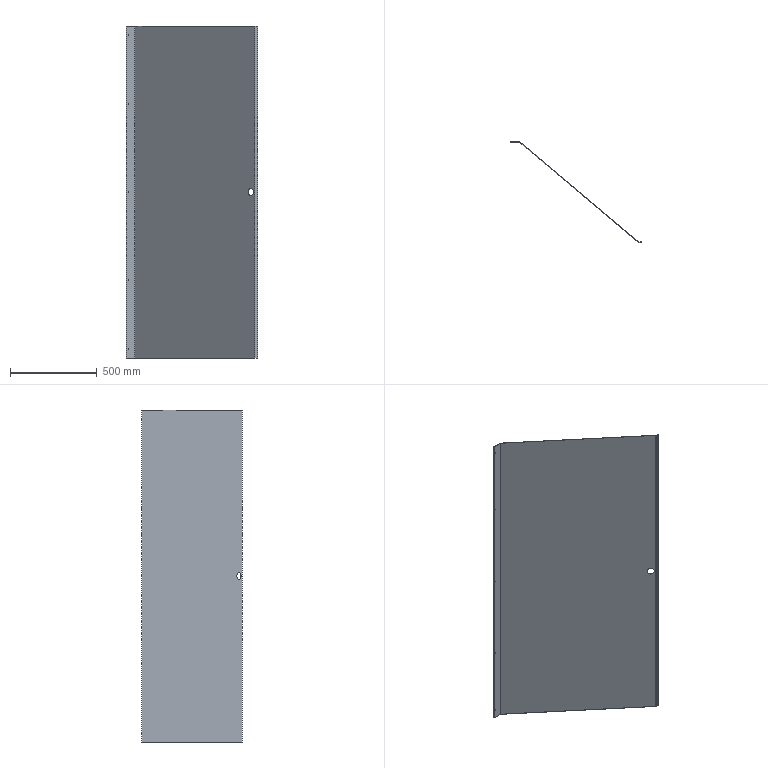Part | SolidWorks | features FlatPattern 1, HoleWzd 1, ICE 1, SMBaseFlange 1, SheetMetal 1 | 1 solid | 34 faces | box 757 x 581.2 x 1915 mm | volume 2223001 mm3 | plane 18 | cylinder 16 | commonest cylinder face diameters 4.5 x10 0.2 x2 2.6 x2 40 x2
STEP:
#1=CARTESIAN_POINT('',(12.,-1.2,47.75));
#2=VERTEX_POINT('',#1);
#3=CARTESIAN_POINT('',(12.,-1.2,52.25));
#4=VERTEX_POINT('',#3);
#5=CARTESIAN_POINT('',(12.,-1.2,50.));
#6=DIRECTION('',(0.,1.,0.));
#7=DIRECTION('',(0.,0.,1.));
#8=AXIS2_PLACEMENT_3D('',#5,#6,#7);
#9=CIRCLE('',#8,2.25);
#10=EDGE_CURVE('',#2,#4,#9,.T.);
#11=ORIENTED_EDGE('',*,*,#10,.F.);
#12=CARTESIAN_POINT('',(12.,0.,47.75));
#13=VERTEX_POINT('',#12);
#14=CARTESIAN_POINT('',(12.,0.,47.75));
#15=DIRECTION('',(0.,1.,0.));
#16=VECTOR('',#15,1000.);
#17=LINE('',#14,#16);
#18=EDGE_CURVE('',#2,#13,#17,.T.);
#19=ORIENTED_EDGE('',*,*,#18,.T.);
#20=CARTESIAN_POINT('',(12.,0.,52.25));
#21=VERTEX_POINT('',#20);
#22=CARTESIAN_POINT('',(12.,0.,50.));
#23=DIRECTION('',(0.,1.,0.));
#24=DIRECTION('',(0.,0.,1.));
#25=AXIS2_PLACEMENT_3D('',#22,#23,#24);
#26=CIRCLE('',#25,2.25);
#27=EDGE_CURVE('',#13,#21,#26,.T.);
#28=ORIENTED_EDGE('',*,*,#27,.T.);
#29=CARTESIAN_POINT('',(12.,0.,52.25));
#30=DIRECTION('',(0.,1.,0.));
#31=VECTOR('',#30,1000.);
#32=LINE('',#29,#31);
#33=EDGE_CURVE('',#4,#21,#32,.T.);
#34=ORIENTED_EDGE('',*,*,#33,.F.);
#35=EDGE_LOOP('',(#11,#19,#28,#34));
#36=FACE_OUTER_BOUND('',#35,.T.);
#37=CARTESIAN_POINT('',(12.,0.,50.));
#38=DIRECTION('',(0.,1.,0.));
#39=DIRECTION('',(0.,0.,1.));
#40=AXIS2_PLACEMENT_3D('',#37,#38,#39);
#41=CYLINDRICAL_SURFACE('',#40,2.25);
#42=ADVANCED_FACE('',(#36),#41,.F.);
#43=CARTESIAN_POINT('',(12.,-1.2,447.75));
#44=VERTEX_POINT('',#43);
#45=CARTESIAN_POINT('',(12.,-1.2,452.25));
#46=VERTEX_POINT('',#45);
#47=CARTESIAN_POINT('',(12.,-1.2,450.));
#48=DIRECTION('',(0.,1.,0.));
#49=DIRECTION('',(0.,0.,1.));
#50=AXIS2_PLACEMENT_3D('',#47,#48,#49);
#51=CIRCLE('',#50,2.25);
#52=EDGE_CURVE('',#44,#46,#51,.T.);
#53=ORIENTED_EDGE('',*,*,#52,.F.);
#54=CARTESIAN_POINT('',(12.,0.,447.75));
#55=VERTEX_POINT('',#54);
#56=CARTESIAN_POINT('',(12.,0.,447.75));
#57=DIRECTION('',(0.,1.,0.));
#58=VECTOR('',#57,1000.);
#59=LINE('',#56,#58);
#60=EDGE_CURVE('',#44,#55,#59,.T.);
#61=ORIENTED_EDGE('',*,*,#60,.T.);
#62=CARTESIAN_POINT('',(12.,0.,452.25));
#63=VERTEX_POINT('',#62);
#64=CARTESIAN_POINT('',(12.,0.,450.));
#65=DIRECTION('',(0.,1.,0.));
#66=DIRECTION('',(0.,0.,1.));
#67=AXIS2_PLACEMENT_3D('',#64,#65,#66);
#68=CIRCLE('',#67,2.25);
#69=EDGE_CURVE('',#55,#63,#68,.T.);
#70=ORIENTED_EDGE('',*,*,#69,.T.);
#71=CARTESIAN_POINT('',(12.,0.,452.25));
#72=DIRECTION('',(0.,1.,0.));
#73=VECTOR('',#72,1000.);
#74=LINE('',#71,#73);
#75=EDGE_CURVE('',#46,#63,#74,.T.);
#76=ORIENTED_EDGE('',*,*,#75,.F.);
#77=EDGE_LOOP('',(#53,#61,#70,#76));
#78=FACE_OUTER_BOUND('',#77,.T.);
#79=CARTESIAN_POINT('',(12.,0.,450.));
#80=DIRECTION('',(0.,1.,0.));
#81=DIRECTION('',(0.,0.,1.));
#82=AXIS2_PLACEMENT_3D('',#79,#80,#81);
#83=CYLINDRICAL_SURFACE('',#82,2.25);
#84=ADVANCED_FACE('',(#78),#83,.F.);
#85=CARTESIAN_POINT('',(12.,-1.2,1462.75));
#86=VERTEX_POINT('',#85);
#87=CARTESIAN_POINT('',(12.,-1.2,1467.25));
#88=VERTEX_POINT('',#87);
#89=CARTESIAN_POINT('',(12.,-1.2,1465.));
#90=DIRECTION('',(0.,1.,0.));
#91=DIRECTION('',(0.,0.,1.));
#92=AXIS2_PLACEMENT_3D('',#89,#90,#91);
#93=CIRCLE('',#92,2.25);
#94=EDGE_CURVE('',#86,#88,#93,.T.);
#95=ORIENTED_EDGE('',*,*,#94,.F.);
#96=CARTESIAN_POINT('',(12.,0.,1462.75));
#97=VERTEX_POINT('',#96);
#98=CARTESIAN_POINT('',(12.,0.,1462.75));
#99=DIRECTION('',(0.,1.,0.));
#100=VECTOR('',#99,1000.);
#101=LINE('',#98,#100);
#102=EDGE_CURVE('',#86,#97,#101,.T.);
#103=ORIENTED_EDGE('',*,*,#102,.T.);
#104=CARTESIAN_POINT('',(12.,0.,1467.25));
#105=VERTEX_POINT('',#104);
#106=CARTESIAN_POINT('',(12.,0.,1465.));
#107=DIRECTION('',(0.,1.,0.));
#108=DIRECTION('',(0.,0.,1.));
#109=AXIS2_PLACEMENT_3D('',#106,#107,#108);
#110=CIRCLE('',#109,2.25);
#111=EDGE_CURVE('',#97,#105,#110,.T.);
#112=ORIENTED_EDGE('',*,*,#111,.T.);
#113=CARTESIAN_POINT('',(12.,0.,1467.25));
#114=DIRECTION('',(0.,1.,0.));
#115=VECTOR('',#114,1000.);
#116=LINE('',#113,#115);
#117=EDGE_CURVE('',#88,#105,#116,.T.);
#118=ORIENTED_EDGE('',*,*,#117,.F.);
#119=EDGE_LOOP('',(#95,#103,#112,#118));
#120=FACE_OUTER_BOUND('',#119,.T.);
#121=CARTESIAN_POINT('',(12.,0.,1465.));
#122=DIRECTION('',(0.,1.,0.));
#123=DIRECTION('',(0.,0.,1.));
#124=AXIS2_PLACEMENT_3D('',#121,#122,#123);
#125=CYLINDRICAL_SURFACE('',#124,2.25);
#126=ADVANCED_FACE('',(#120),#125,.F.);
#127=CARTESIAN_POINT('',(12.,-1.2,1862.75));
#128=VERTEX_POINT('',#127);
#129=CARTESIAN_POINT('',(12.,-1.2,1867.25));
#130=VERTEX_POINT('',#129);
#131=CARTESIAN_POINT('',(12.,-1.2,1865.));
#132=DIRECTION('',(0.,1.,0.));
#133=DIRECTION('',(0.,0.,1.));
#134=AXIS2_PLACEMENT_3D('',#131,#132,#133);
#135=CIRCLE('',#134,2.25);
#136=EDGE_CURVE('',#128,#130,#135,.T.);
#137=ORIENTED_EDGE('',*,*,#136,.F.);
#138=CARTESIAN_POINT('',(12.,0.,1862.75));
#139=VERTEX_POINT('',#138);
#140=CARTESIAN_POINT('',(12.,0.,1862.75));
#141=DIRECTION('',(0.,1.,0.));
#142=VECTOR('',#141,1000.);
#143=LINE('',#140,#142);
#144=EDGE_CURVE('',#128,#139,#143,.T.);
#145=ORIENTED_EDGE('',*,*,#144,.T.);
#146=CARTESIAN_POINT('',(12.,0.,1867.25));
#147=VERTEX_POINT('',#146);
#148=CARTESIAN_POINT('',(12.,0.,1865.));
#149=DIRECTION('',(0.,1.,0.));
#150=DIRECTION('',(0.,0.,1.));
#151=AXIS2_PLACEMENT_3D('',#148,#149,#150);
#152=CIRCLE('',#151,2.25);
#153=EDGE_CURVE('',#139,#147,#152,.T.);
#154=ORIENTED_EDGE('',*,*,#153,.T.);
#155=CARTESIAN_POINT('',(12.,0.,1867.25));
#156=DIRECTION('',(0.,1.,0.));
#157=VECTOR('',#156,1000.);
#158=LINE('',#155,#157);
#159=EDGE_CURVE('',#130,#147,#158,.T.);
#160=ORIENTED_EDGE('',*,*,#159,.F.);
#161=EDGE_LOOP('',(#137,#145,#154,#160));
#162=FACE_OUTER_BOUND('',#161,.T.);
#163=CARTESIAN_POINT('',(12.,0.,1865.));
#164=DIRECTION('',(0.,1.,0.));
#165=DIRECTION('',(0.,0.,1.));
#166=AXIS2_PLACEMENT_3D('',#163,#164,#165);
#167=CYLINDRICAL_SURFACE('',#166,2.25);
#168=ADVANCED_FACE('',(#162),#167,.F.);
#169=CARTESIAN_POINT('',(12.,-1.2,955.25));
#170=VERTEX_POINT('',#169);
#171=CARTESIAN_POINT('',(12.,-1.2,959.75));
#172=VERTEX_POINT('',#171);
#173=CARTESIAN_POINT('',(12.,-1.2,957.5));
#174=DIRECTION('',(0.,1.,0.));
#175=DIRECTION('',(0.,0.,1.));
#176=AXIS2_PLACEMENT_3D('',#173,#174,#175);
#177=CIRCLE('',#176,2.25);
#178=EDGE_CURVE('',#170,#172,#177,.T.);
#179=ORIENTED_EDGE('',*,*,#178,.F.);
#180=CARTESIAN_POINT('',(12.,0.,955.25));
#181=VERTEX_POINT('',#180);
#182=CARTESIAN_POINT('',(12.,0.,955.25));
#183=DIRECTION('',(0.,1.,0.));
#184=VECTOR('',#183,1000.);
#185=LINE('',#182,#184);
#186=EDGE_CURVE('',#170,#181,#185,.T.);
#187=ORIENTED_EDGE('',*,*,#186,.T.);
#188=CARTESIAN_POINT('',(12.,0.,959.75));
#189=VERTEX_POINT('',#188);
#190=CARTESIAN_POINT('',(12.,0.,957.5));
#191=DIRECTION('',(0.,1.,0.));
#192=DIRECTION('',(0.,0.,1.));
#193=AXIS2_PLACEMENT_3D('',#190,#191,#192);
#194=CIRCLE('',#193,2.25);
#195=EDGE_CURVE('',#181,#189,#194,.T.);
#196=ORIENTED_EDGE('',*,*,#195,.T.);
#197=CARTESIAN_POINT('',(12.,0.,959.75));
#198=DIRECTION('',(0.,1.,0.));
#199=VECTOR('',#198,1000.);
#200=LINE('',#197,#199);
#201=EDGE_CURVE('',#172,#189,#200,.T.);
#202=ORIENTED_EDGE('',*,*,#201,.F.);
#203=EDGE_LOOP('',(#179,#187,#196,#202));
#204=FACE_OUTER_BOUND('',#203,.T.);
#205=CARTESIAN_POINT('',(12.,0.,957.5));
#206=DIRECTION('',(0.,1.,0.));
#207=DIRECTION('',(0.,0.,1.));
#208=AXIS2_PLACEMENT_3D('',#205,#206,#207);
#209=CYLINDRICAL_SURFACE('',#208,2.25);
#210=ADVANCED_FACE('',(#204),#209,.F.);
#211=CARTESIAN_POINT('',(732.807,-574.509,957.5));
#212=VERTEX_POINT('',#211);
#213=CARTESIAN_POINT('',(702.165,-548.798,957.5));
#214=VERTEX_POINT('',#213);
#215=CARTESIAN_POINT('',(717.486,-561.654,957.5));
#216=DIRECTION('',(0.6428,0.766,0.));
#217=DIRECTION('',(-0.766,0.6428,0.));
#218=AXIS2_PLACEMENT_3D('',#215,#216,#217);
#219=CIRCLE('',#218,20.);
#220=EDGE_CURVE('',#212,#214,#219,.T.);
#221=ORIENTED_EDGE('',*,*,#220,.F.);
#222=CARTESIAN_POINT('',(733.578,-573.59,957.5));
#223=VERTEX_POINT('',#222);
#224=CARTESIAN_POINT('',(727.15,-581.25,957.5));
#225=DIRECTION('',(0.6428,0.766,0.));
#226=VECTOR('',#225,1000.);
#227=LINE('',#224,#226);
#228=EDGE_CURVE('',#212,#223,#227,.T.);
#229=ORIENTED_EDGE('',*,*,#228,.T.);
#230=CARTESIAN_POINT('',(702.936,-547.879,957.5));
#231=VERTEX_POINT('',#230);
#232=CARTESIAN_POINT('',(718.257,-560.734,957.5));
#233=DIRECTION('',(0.6428,0.766,0.));
#234=DIRECTION('',(-0.766,0.6428,0.));
#235=AXIS2_PLACEMENT_3D('',#232,#233,#234);
#236=CIRCLE('',#235,20.);
#237=EDGE_CURVE('',#223,#231,#236,.T.);
#238=ORIENTED_EDGE('',*,*,#237,.T.);
#239=CARTESIAN_POINT('',(696.508,-555.539,957.5));
#240=DIRECTION('',(0.6428,0.766,0.));
#241=VECTOR('',#240,1000.);
#242=LINE('',#239,#241);
#243=EDGE_CURVE('',#214,#231,#242,.T.);
#244=ORIENTED_EDGE('',*,*,#243,.F.);
#245=EDGE_LOOP('',(#221,#229,#238,#244));
#246=FACE_OUTER_BOUND('',#245,.T.);
#247=CARTESIAN_POINT('',(711.829,-568.395,957.5));
#248=DIRECTION('',(0.6428,0.766,0.));
#249=DIRECTION('',(-0.766,0.6428,0.));
#250=AXIS2_PLACEMENT_3D('',#247,#248,#249);
#251=CYLINDRICAL_SURFACE('',#250,20.);
#252=ADVANCED_FACE('',(#246),#251,.F.);
#253=CARTESIAN_POINT('',(50.362,-0.3041,1915.));
#254=VERTEX_POINT('',#253);
#255=CARTESIAN_POINT('',(49.591,-1.223,1915.));
#256=VERTEX_POINT('',#255);
#257=CARTESIAN_POINT('',(50.362,-0.3041,1915.));
#258=DIRECTION('',(-0.6428,-0.766,0.));
#259=VECTOR('',#258,1000.);
#260=LINE('',#257,#259);
#261=EDGE_CURVE('',#254,#256,#260,.T.);
#262=ORIENTED_EDGE('',*,*,#261,.F.);
#263=CARTESIAN_POINT('',(49.527,0.,1915.));
#264=VERTEX_POINT('',#263);
#265=CARTESIAN_POINT('',(49.527,-1.3,1915.));
#266=DIRECTION('',(0.,0.,-1.));
#267=DIRECTION('',(1.,0.,0.));
#268=AXIS2_PLACEMENT_3D('',#265,#266,#267);
#269=CIRCLE('',#268,1.3);
#270=EDGE_CURVE('',#264,#254,#269,.T.);
#271=ORIENTED_EDGE('',*,*,#270,.F.);
#272=CARTESIAN_POINT('',(49.527,-1.2,1915.));
#273=VERTEX_POINT('',#272);
#274=CARTESIAN_POINT('',(49.527,-1.2,1915.));
#275=DIRECTION('',(0.,1.,0.));
#276=VECTOR('',#275,1000.);
#277=LINE('',#274,#276);
#278=EDGE_CURVE('',#273,#264,#277,.T.);
#279=ORIENTED_EDGE('',*,*,#278,.F.);
#280=CARTESIAN_POINT('',(49.527,-1.3,1915.));
#281=DIRECTION('',(0.,0.,-1.));
#282=DIRECTION('',(1.,0.,0.));
#283=AXIS2_PLACEMENT_3D('',#280,#281,#282);
#284=CIRCLE('',#283,0.1);
#285=EDGE_CURVE('',#273,#256,#284,.T.);
#286=ORIENTED_EDGE('',*,*,#285,.T.);
#287=EDGE_LOOP('',(#262,#271,#279,#286));
#288=FACE_OUTER_BOUND('',#287,.T.);
#289=CARTESIAN_POINT('',(50.362,-0.3041,1915.));
#290=DIRECTION('',(0.,0.,1.));
#291=DIRECTION('',(1.,0.,0.));
#292=AXIS2_PLACEMENT_3D('',#289,#290,#291);
#293=PLANE('',#292);
#294=ADVANCED_FACE('',(#288),#293,.T.);
#295=CARTESIAN_POINT('',(741.189,-579.977,1915.));
#296=VERTEX_POINT('',#295);
#297=CARTESIAN_POINT('',(50.,0.,1915.));
#298=DIRECTION('',(0.766,-0.6428,0.));
#299=VECTOR('',#298,1000.);
#300=LINE('',#297,#299);
#301=EDGE_CURVE('',#254,#296,#300,.T.);
#302=ORIENTED_EDGE('',*,*,#301,.F.);
#303=ORIENTED_EDGE('',*,*,#261,.T.);
#304=CARTESIAN_POINT('',(740.418,-580.896,1915.));
#305=VERTEX_POINT('',#304);
#306=CARTESIAN_POINT('',(49.229,-0.9193,1915.));
#307=DIRECTION('',(0.766,-0.6428,0.));
#308=VECTOR('',#307,1000.);
#309=LINE('',#306,#308);
#310=EDGE_CURVE('',#256,#305,#309,.T.);
#311=ORIENTED_EDGE('',*,*,#310,.T.);
#312=CARTESIAN_POINT('',(740.418,-580.896,1915.));
#313=DIRECTION('',(0.6428,0.766,0.));
#314=VECTOR('',#313,1000.);
#315=LINE('',#312,#314);
#316=EDGE_CURVE('',#305,#296,#315,.T.);
#317=ORIENTED_EDGE('',*,*,#316,.T.);
#318=EDGE_LOOP('',(#302,#303,#311,#317));
#319=FACE_OUTER_BOUND('',#318,.T.);
#320=CARTESIAN_POINT('',(49.527,-1.2,1915.));
#321=DIRECTION('',(0.,0.,1.));
#322=DIRECTION('',(1.,0.,0.));
#323=AXIS2_PLACEMENT_3D('',#320,#321,#322);
#324=PLANE('',#323);
#325=ADVANCED_FACE('',(#319),#324,.T.);
#326=CARTESIAN_POINT('',(49.527,0.,0.));
#327=VERTEX_POINT('',#326);
#328=CARTESIAN_POINT('',(49.527,-1.2,0.));
#329=VERTEX_POINT('',#328);
#330=CARTESIAN_POINT('',(49.527,0.,0.));
#331=DIRECTION('',(0.,-1.,0.));
#332=VECTOR('',#331,1000.);
#333=LINE('',#330,#332);
#334=EDGE_CURVE('',#327,#329,#333,.T.);
#335=ORIENTED_EDGE('',*,*,#334,.F.);
#336=CARTESIAN_POINT('',(50.362,-0.3041,0.));
#337=VERTEX_POINT('',#336);
#338=CARTESIAN_POINT('',(49.527,-1.3,0.));
#339=DIRECTION('',(0.,0.,-1.));
#340=DIRECTION('',(1.,0.,0.));
#341=AXIS2_PLACEMENT_3D('',#338,#339,#340);
#342=CIRCLE('',#341,1.3);
#343=EDGE_CURVE('',#327,#337,#342,.T.);
#344=ORIENTED_EDGE('',*,*,#343,.T.);
#345=CARTESIAN_POINT('',(49.591,-1.223,0.));
#346=VERTEX_POINT('',#345);
#347=CARTESIAN_POINT('',(49.591,-1.223,0.));
#348=DIRECTION('',(0.6428,0.766,0.));
#349=VECTOR('',#348,1000.);
#350=LINE('',#347,#349);
#351=EDGE_CURVE('',#346,#337,#350,.T.);
#352=ORIENTED_EDGE('',*,*,#351,.F.);
#353=CARTESIAN_POINT('',(49.527,-1.3,0.));
#354=DIRECTION('',(0.,0.,-1.));
#355=DIRECTION('',(1.,0.,0.));
#356=AXIS2_PLACEMENT_3D('',#353,#354,#355);
#357=CIRCLE('',#356,0.1);
#358=EDGE_CURVE('',#329,#346,#357,.T.);
#359=ORIENTED_EDGE('',*,*,#358,.F.);
#360=EDGE_LOOP('',(#335,#344,#352,#359));
#361=FACE_OUTER_BOUND('',#360,.T.);
#362=CARTESIAN_POINT('',(49.527,0.,0.));
#363=DIRECTION('',(0.,0.,-1.));
#364=DIRECTION('',(-1.,0.,0.));
#365=AXIS2_PLACEMENT_3D('',#362,#363,#364);
#366=PLANE('',#365);
#367=ADVANCED_FACE('',(#361),#366,.T.);
#368=CARTESIAN_POINT('',(0.,0.,0.));
#369=VERTEX_POINT('',#368);
#370=CARTESIAN_POINT('',(0.,0.,0.));
#371=DIRECTION('',(1.,0.,0.));
#372=VECTOR('',#371,1000.);
#373=LINE('',#370,#372);
#374=EDGE_CURVE('',#369,#327,#373,.T.);
#375=ORIENTED_EDGE('',*,*,#374,.T.);
#376=ORIENTED_EDGE('',*,*,#334,.T.);
#377=CARTESIAN_POINT('',(0.,-1.2,0.));
#378=VERTEX_POINT('',#377);
#379=CARTESIAN_POINT('',(0.,-1.2,0.));
#380=DIRECTION('',(1.,0.,0.));
#381=VECTOR('',#380,1000.);
#382=LINE('',#379,#381);
#383=EDGE_CURVE('',#378,#329,#382,.T.);
#384=ORIENTED_EDGE('',*,*,#383,.F.);
#385=CARTESIAN_POINT('',(0.,-1.2,0.));
#386=DIRECTION('',(0.,1.,0.));
#387=VECTOR('',#386,1000.);
#388=LINE('',#385,#387);
#389=EDGE_CURVE('',#378,#369,#388,.T.);
#390=ORIENTED_EDGE('',*,*,#389,.T.);
#391=EDGE_LOOP('',(#375,#376,#384,#390));
#392=FACE_OUTER_BOUND('',#391,.T.);
#393=CARTESIAN_POINT('',(49.591,-1.223,0.));
#394=DIRECTION('',(0.,0.,-1.));
#395=DIRECTION('',(-1.,0.,0.));
#396=AXIS2_PLACEMENT_3D('',#393,#394,#395);
#397=PLANE('',#396);
#398=ADVANCED_FACE('',(#392),#397,.T.);
#399=CARTESIAN_POINT('',(741.253,-580.,1915.));
#400=VERTEX_POINT('',#399);
#401=CARTESIAN_POINT('',(741.253,-581.2,1915.));
#402=VERTEX_POINT('',#401);
#403=CARTESIAN_POINT('',(741.253,-580.,1915.));
#404=DIRECTION('',(0.,-1.,0.));
#405=VECTOR('',#404,1000.);
#406=LINE('',#403,#405);
#407=EDGE_CURVE('',#400,#402,#406,.T.);
#408=ORIENTED_EDGE('',*,*,#407,.F.);
#409=CARTESIAN_POINT('',(741.253,-579.9,1915.));
#410=DIRECTION('',(0.,0.,1.));
#411=DIRECTION('',(-1.,0.,0.));
#412=AXIS2_PLACEMENT_3D('',#409,#410,#411);
#413=CIRCLE('',#412,0.1);
#414=EDGE_CURVE('',#296,#400,#413,.T.);
#415=ORIENTED_EDGE('',*,*,#414,.F.);
#416=ORIENTED_EDGE('',*,*,#316,.F.);
#417=CARTESIAN_POINT('',(741.253,-579.9,1915.));
#418=DIRECTION('',(0.,0.,1.));
#419=DIRECTION('',(1.,0.,0.));
#420=AXIS2_PLACEMENT_3D('',#417,#418,#419);
#421=CIRCLE('',#420,1.3);
#422=EDGE_CURVE('',#305,#402,#421,.T.);
#423=ORIENTED_EDGE('',*,*,#422,.T.);
#424=EDGE_LOOP('',(#408,#415,#416,#423));
#425=FACE_OUTER_BOUND('',#424,.T.);
#426=CARTESIAN_POINT('',(741.253,-580.,1915.));
#427=DIRECTION('',(0.,0.,1.));
#428=DIRECTION('',(1.,0.,0.));
#429=AXIS2_PLACEMENT_3D('',#426,#427,#428);
#430=PLANE('',#429);
#431=ADVANCED_FACE('',(#425),#430,.T.);
#432=CARTESIAN_POINT('',(757.,-580.,1915.));
#433=VERTEX_POINT('',#432);
#434=CARTESIAN_POINT('',(741.217,-580.,1915.));
#435=DIRECTION('',(1.,0.,0.));
#436=VECTOR('',#435,1000.);
#437=LINE('',#434,#436);
#438=EDGE_CURVE('',#400,#433,#437,.T.);
#439=ORIENTED_EDGE('',*,*,#438,.F.);
#440=ORIENTED_EDGE('',*,*,#407,.T.);
#441=CARTESIAN_POINT('',(757.,-581.2,1915.));
#442=VERTEX_POINT('',#441);
#443=CARTESIAN_POINT('',(741.217,-581.2,1915.));
#444=DIRECTION('',(1.,0.,0.));
#445=VECTOR('',#444,1000.);
#446=LINE('',#443,#445);
#447=EDGE_CURVE('',#402,#442,#446,.T.);
#448=ORIENTED_EDGE('',*,*,#447,.T.);
#449=CARTESIAN_POINT('',(757.,-580.,1915.));
#450=DIRECTION('',(0.,-1.,0.));
#451=VECTOR('',#450,1000.);
#452=LINE('',#449,#451);
#453=EDGE_CURVE('',#433,#442,#452,.T.);
#454=ORIENTED_EDGE('',*,*,#453,.F.);
#455=EDGE_LOOP('',(#439,#440,#448,#454));
#456=FACE_OUTER_BOUND('',#455,.T.);
#457=CARTESIAN_POINT('',(740.418,-580.896,1915.));
#458=DIRECTION('',(0.,0.,1.));
#459=DIRECTION('',(1.,0.,0.));
#460=AXIS2_PLACEMENT_3D('',#457,#458,#459);
#461=PLANE('',#460);
#462=ADVANCED_FACE('',(#456),#461,.T.);
#463=CARTESIAN_POINT('',(741.189,-579.977,0.));
#464=VERTEX_POINT('',#463);
#465=CARTESIAN_POINT('',(740.418,-580.896,0.));
#466=VERTEX_POINT('',#465);
#467=CARTESIAN_POINT('',(741.189,-579.977,0.));
#468=DIRECTION('',(-0.6428,-0.766,0.));
#469=VECTOR('',#468,1000.);
#470=LINE('',#467,#469);
#471=EDGE_CURVE('',#464,#466,#470,.T.);
#472=ORIENTED_EDGE('',*,*,#471,.F.);
#473=CARTESIAN_POINT('',(741.253,-580.,0.));
#474=VERTEX_POINT('',#473);
#475=CARTESIAN_POINT('',(741.253,-579.9,0.));
#476=DIRECTION('',(0.,0.,1.));
#477=DIRECTION('',(-1.,0.,0.));
#478=AXIS2_PLACEMENT_3D('',#475,#476,#477);
#479=CIRCLE('',#478,0.1);
#480=EDGE_CURVE('',#464,#474,#479,.T.);
#481=ORIENTED_EDGE('',*,*,#480,.T.);
#482=CARTESIAN_POINT('',(741.253,-581.2,0.));
#483=VERTEX_POINT('',#482);
#484=CARTESIAN_POINT('',(741.253,-581.2,0.));
#485=DIRECTION('',(0.,1.,0.));
#486=VECTOR('',#485,1000.);
#487=LINE('',#484,#486);
#488=EDGE_CURVE('',#483,#474,#487,.T.);
#489=ORIENTED_EDGE('',*,*,#488,.F.);
#490=CARTESIAN_POINT('',(741.253,-579.9,0.));
#491=DIRECTION('',(0.,0.,1.));
#492=DIRECTION('',(1.,0.,0.));
#493=AXIS2_PLACEMENT_3D('',#490,#491,#492);
#494=CIRCLE('',#493,1.3);
#495=EDGE_CURVE('',#466,#483,#494,.T.);
#496=ORIENTED_EDGE('',*,*,#495,.F.);
#497=EDGE_LOOP('',(#472,#481,#489,#496));
#498=FACE_OUTER_BOUND('',#497,.T.);
#499=CARTESIAN_POINT('',(741.189,-579.977,0.));
#500=DIRECTION('',(0.,0.,-1.));
#501=DIRECTION('',(-1.,0.,0.));
#502=AXIS2_PLACEMENT_3D('',#499,#500,#501);
#503=PLANE('',#502);
#504=ADVANCED_FACE('',(#498),#503,.T.);
#505=CARTESIAN_POINT('',(50.,0.,0.));
#506=DIRECTION('',(0.766,-0.6428,0.));
#507=VECTOR('',#506,1000.);
#508=LINE('',#505,#507);
#509=EDGE_CURVE('',#337,#464,#508,.T.);
#510=ORIENTED_EDGE('',*,*,#509,.T.);
#511=ORIENTED_EDGE('',*,*,#471,.T.);
#512=CARTESIAN_POINT('',(49.229,-0.9193,0.));
#513=DIRECTION('',(0.766,-0.6428,0.));
#514=VECTOR('',#513,1000.);
#515=LINE('',#512,#514);
#516=EDGE_CURVE('',#346,#466,#515,.T.);
#517=ORIENTED_EDGE('',*,*,#516,.F.);
#518=ORIENTED_EDGE('',*,*,#351,.T.);
#519=EDGE_LOOP('',(#510,#511,#517,#518));
#520=FACE_OUTER_BOUND('',#519,.T.);
#521=CARTESIAN_POINT('',(741.253,-581.2,0.));
#522=DIRECTION('',(0.,0.,-1.));
#523=DIRECTION('',(-1.,0.,0.));
#524=AXIS2_PLACEMENT_3D('',#521,#522,#523);
#525=PLANE('',#524);
#526=ADVANCED_FACE('',(#520),#525,.T.);
#527=CARTESIAN_POINT('',(757.,-581.2,0.));
#528=VERTEX_POINT('',#527);
#529=CARTESIAN_POINT('',(741.217,-581.2,0.));
#530=DIRECTION('',(1.,0.,0.));
#531=VECTOR('',#530,1000.);
#532=LINE('',#529,#531);
#533=EDGE_CURVE('',#483,#528,#532,.T.);
#534=ORIENTED_EDGE('',*,*,#533,.T.);
#535=CARTESIAN_POINT('',(757.,-581.2,1915.));
#536=DIRECTION('',(0.,0.,-1.));
#537=VECTOR('',#536,1000.);
#538=LINE('',#535,#537);
#539=EDGE_CURVE('',#442,#528,#538,.T.);
#540=ORIENTED_EDGE('',*,*,#539,.F.);
#541=ORIENTED_EDGE('',*,*,#447,.F.);
#542=CARTESIAN_POINT('',(741.253,-581.2,1915.));
#543=DIRECTION('',(0.,0.,-1.));
#544=VECTOR('',#543,1000.);
#545=LINE('',#542,#544);
#546=EDGE_CURVE('',#402,#483,#545,.T.);
#547=ORIENTED_EDGE('',*,*,#546,.T.);
#548=EDGE_LOOP('',(#534,#540,#541,#547));
#549=FACE_OUTER_BOUND('',#548,.T.);
#550=CARTESIAN_POINT('',(741.217,-581.2,1915.));
#551=DIRECTION('',(0.,1.,0.));
#552=DIRECTION('',(0.,0.,1.));
#553=AXIS2_PLACEMENT_3D('',#550,#551,#552);
#554=PLANE('',#553);
#555=ADVANCED_FACE('',(#549),#554,.F.);
#556=CARTESIAN_POINT('',(757.,-580.,0.));
#557=VERTEX_POINT('',#556);
#558=CARTESIAN_POINT('',(757.,-580.,0.));
#559=DIRECTION('',(0.,-1.,0.));
#560=VECTOR('',#559,1000.);
#561=LINE('',#558,#560);
#562=EDGE_CURVE('',#557,#528,#561,.T.);
#563=ORIENTED_EDGE('',*,*,#562,.F.);
#564=CARTESIAN_POINT('',(757.,-580.,1915.));
#565=DIRECTION('',(0.,0.,-1.));
#566=VECTOR('',#565,1000.);
#567=LINE('',#564,#566);
#568=EDGE_CURVE('',#433,#557,#567,.T.);
#569=ORIENTED_EDGE('',*,*,#568,.F.);
#570=ORIENTED_EDGE('',*,*,#453,.T.);
#571=ORIENTED_EDGE('',*,*,#539,.T.);
#572=EDGE_LOOP('',(#563,#569,#570,#571));
#573=FACE_OUTER_BOUND('',#572,.T.);
#574=CARTESIAN_POINT('',(757.,-580.,1915.));
#575=DIRECTION('',(1.,0.,0.));
#576=DIRECTION('',(0.,0.,-1.));
#577=AXIS2_PLACEMENT_3D('',#574,#575,#576);
#578=PLANE('',#577);
#579=ADVANCED_FACE('',(#573),#578,.T.);
#580=CARTESIAN_POINT('',(741.217,-580.,0.));
#581=DIRECTION('',(1.,0.,0.));
#582=VECTOR('',#581,1000.);
#583=LINE('',#580,#582);
#584=EDGE_CURVE('',#474,#557,#583,.T.);
#585=ORIENTED_EDGE('',*,*,#584,.F.);
#586=CARTESIAN_POINT('',(741.253,-580.,1915.));
#587=DIRECTION('',(0.,0.,-1.));
#588=VECTOR('',#587,1000.);
#589=LINE('',#586,#588);
#590=EDGE_CURVE('',#400,#474,#589,.T.);
#591=ORIENTED_EDGE('',*,*,#590,.F.);
#592=ORIENTED_EDGE('',*,*,#438,.T.);
#593=ORIENTED_EDGE('',*,*,#568,.T.);
#594=EDGE_LOOP('',(#585,#591,#592,#593));
#595=FACE_OUTER_BOUND('',#594,.T.);
#596=CARTESIAN_POINT('',(741.217,-580.,1915.));
#597=DIRECTION('',(0.,1.,0.));
#598=DIRECTION('',(0.,0.,1.));
#599=AXIS2_PLACEMENT_3D('',#596,#597,#598);
#600=PLANE('',#599);
#601=ADVANCED_FACE('',(#595),#600,.T.);
#602=ORIENTED_EDGE('',*,*,#480,.F.);
#603=CARTESIAN_POINT('',(741.189,-579.977,1915.));
#604=DIRECTION('',(0.,0.,-1.));
#605=VECTOR('',#604,1000.);
#606=LINE('',#603,#605);
#607=EDGE_CURVE('',#296,#464,#606,.T.);
#608=ORIENTED_EDGE('',*,*,#607,.F.);
#609=ORIENTED_EDGE('',*,*,#414,.T.);
#610=ORIENTED_EDGE('',*,*,#590,.T.);
#611=EDGE_LOOP('',(#602,#608,#609,#610));
#612=FACE_OUTER_BOUND('',#611,.T.);
#613=CARTESIAN_POINT('',(741.253,-579.9,1915.));
#614=DIRECTION('',(0.,0.,-1.));
#615=DIRECTION('',(-1.,0.,0.));
#616=AXIS2_PLACEMENT_3D('',#613,#614,#615);
#617=CYLINDRICAL_SURFACE('',#616,0.1);
#618=ADVANCED_FACE('',(#612),#617,.F.);
#619=CARTESIAN_POINT('',(718.257,-560.734,957.5));
#620=DIRECTION('',(0.6428,0.766,0.));
#621=DIRECTION('',(-0.766,0.6428,0.));
#622=AXIS2_PLACEMENT_3D('',#619,#620,#621);
#623=CIRCLE('',#622,20.);
#624=EDGE_CURVE('',#231,#223,#623,.T.);
#625=ORIENTED_EDGE('',*,*,#624,.F.);
#626=ORIENTED_EDGE('',*,*,#237,.F.);
#627=EDGE_LOOP('',(#625,#626));
#628=FACE_BOUND('',#627,.T.);
#629=ORIENTED_EDGE('',*,*,#509,.F.);
#630=CARTESIAN_POINT('',(50.362,-0.3041,1915.));
#631=DIRECTION('',(0.,0.,-1.));
#632=VECTOR('',#631,1000.);
#633=LINE('',#630,#632);
#634=EDGE_CURVE('',#254,#337,#633,.T.);
#635=ORIENTED_EDGE('',*,*,#634,.F.);
#636=ORIENTED_EDGE('',*,*,#301,.T.);
#637=ORIENTED_EDGE('',*,*,#607,.T.);
#638=EDGE_LOOP('',(#629,#635,#636,#637));
#639=FACE_OUTER_BOUND('',#638,.T.);
#640=CARTESIAN_POINT('',(50.,0.,1915.));
#641=DIRECTION('',(0.6428,0.766,0.));
#642=DIRECTION('',(-0.766,0.6428,0.));
#643=AXIS2_PLACEMENT_3D('',#640,#641,#642);
#644=PLANE('',#643);
#645=ADVANCED_FACE('',(#628,#639),#644,.T.);
#646=ORIENTED_EDGE('',*,*,#343,.F.);
#647=CARTESIAN_POINT('',(49.527,0.,1915.));
#648=DIRECTION('',(0.,0.,-1.));
#649=VECTOR('',#648,1000.);
#650=LINE('',#647,#649);
#651=EDGE_CURVE('',#264,#327,#650,.T.);
#652=ORIENTED_EDGE('',*,*,#651,.F.);
#653=ORIENTED_EDGE('',*,*,#270,.T.);
#654=ORIENTED_EDGE('',*,*,#634,.T.);
#655=EDGE_LOOP('',(#646,#652,#653,#654));
#656=FACE_OUTER_BOUND('',#655,.T.);
#657=CARTESIAN_POINT('',(49.527,-1.3,1915.));
#658=DIRECTION('',(0.,0.,-1.));
#659=DIRECTION('',(-1.,0.,0.));
#660=AXIS2_PLACEMENT_3D('',#657,#658,#659);
#661=CYLINDRICAL_SURFACE('',#660,1.3);
#662=ADVANCED_FACE('',(#656),#661,.T.);
#663=CARTESIAN_POINT('',(12.,0.,50.));
#664=DIRECTION('',(0.,1.,0.));
#665=DIRECTION('',(0.,0.,1.));
#666=AXIS2_PLACEMENT_3D('',#663,#664,#665);
#667=CIRCLE('',#666,2.25);
#668=EDGE_CURVE('',#21,#13,#667,.T.);
#669=ORIENTED_EDGE('',*,*,#668,.F.);
#670=ORIENTED_EDGE('',*,*,#27,.F.);
#671=EDGE_LOOP('',(#669,#670));
#672=FACE_BOUND('',#671,.T.);
#673=CARTESIAN_POINT('',(12.,0.,450.));
#674=DIRECTION('',(0.,1.,0.));
#675=DIRECTION('',(0.,0.,1.));
#676=AXIS2_PLACEMENT_3D('',#673,#674,#675);
#677=CIRCLE('',#676,2.25);
#678=EDGE_CURVE('',#63,#55,#677,.T.);
#679=ORIENTED_EDGE('',*,*,#678,.F.);
#680=ORIENTED_EDGE('',*,*,#69,.F.);
#681=EDGE_LOOP('',(#679,#680));
#682=FACE_BOUND('',#681,.T.);
#683=CARTESIAN_POINT('',(12.,0.,1465.));
#684=DIRECTION('',(0.,1.,0.));
#685=DIRECTION('',(0.,0.,1.));
#686=AXIS2_PLACEMENT_3D('',#683,#684,#685);
#687=CIRCLE('',#686,2.25);
#688=EDGE_CURVE('',#105,#97,#687,.T.);
#689=ORIENTED_EDGE('',*,*,#688,.F.);
#690=ORIENTED_EDGE('',*,*,#111,.F.);
#691=EDGE_LOOP('',(#689,#690));
#692=FACE_BOUND('',#691,.T.);
#693=CARTESIAN_POINT('',(12.,0.,1865.));
#694=DIRECTION('',(0.,1.,0.));
#695=DIRECTION('',(0.,0.,1.));
#696=AXIS2_PLACEMENT_3D('',#693,#694,#695);
#697=CIRCLE('',#696,2.25);
#698=EDGE_CURVE('',#147,#139,#697,.T.);
#699=ORIENTED_EDGE('',*,*,#698,.F.);
#700=ORIENTED_EDGE('',*,*,#153,.F.);
#701=EDGE_LOOP('',(#699,#700));
#702=FACE_BOUND('',#701,.T.);
#703=CARTESIAN_POINT('',(12.,0.,957.5));
#704=DIRECTION('',(0.,1.,0.));
#705=DIRECTION('',(0.,0.,1.));
#706=AXIS2_PLACEMENT_3D('',#703,#704,#705);
#707=CIRCLE('',#706,2.25);
#708=EDGE_CURVE('',#189,#181,#707,.T.);
#709=ORIENTED_EDGE('',*,*,#708,.F.);
#710=ORIENTED_EDGE('',*,*,#195,.F.);
#711=EDGE_LOOP('',(#709,#710));
#712=FACE_BOUND('',#711,.T.);
#713=ORIENTED_EDGE('',*,*,#374,.F.);
#714=CARTESIAN_POINT('',(0.,0.,1915.));
#715=VERTEX_POINT('',#714);
#716=CARTESIAN_POINT('',(0.,0.,1915.));
#717=DIRECTION('',(0.,0.,-1.));
#718=VECTOR('',#717,1000.);
#719=LINE('',#716,#718);
#720=EDGE_CURVE('',#715,#369,#719,.T.);
#721=ORIENTED_EDGE('',*,*,#720,.F.);
#722=CARTESIAN_POINT('',(0.,0.,1915.));
#723=DIRECTION('',(1.,0.,0.));
#724=VECTOR('',#723,1000.);
#725=LINE('',#722,#724);
#726=EDGE_CURVE('',#715,#264,#725,.T.);
#727=ORIENTED_EDGE('',*,*,#726,.T.);
#728=ORIENTED_EDGE('',*,*,#651,.T.);
#729=EDGE_LOOP('',(#713,#721,#727,#728));
#730=FACE_OUTER_BOUND('',#729,.T.);
#731=CARTESIAN_POINT('',(0.,0.,1915.));
#732=DIRECTION('',(0.,1.,0.));
#733=DIRECTION('',(0.,0.,1.));
#734=AXIS2_PLACEMENT_3D('',#731,#732,#733);
#735=PLANE('',#734);
#736=ADVANCED_FACE('',(#672,#682,#692,#702,#712,#730),#735,.T.);
#737=ORIENTED_EDGE('',*,*,#389,.F.);
#738=CARTESIAN_POINT('',(0.,-1.2,1915.));
#739=VERTEX_POINT('',#738);
#740=CARTESIAN_POINT('',(0.,-1.2,1915.));
#741=DIRECTION('',(0.,0.,-1.));
#742=VECTOR('',#741,1000.);
#743=LINE('',#740,#742);
#744=EDGE_CURVE('',#739,#378,#743,.T.);
#745=ORIENTED_EDGE('',*,*,#744,.F.);
#746=CARTESIAN_POINT('',(0.,-1.2,1915.));
#747=DIRECTION('',(0.,1.,0.));
#748=VECTOR('',#747,1000.);
#749=LINE('',#746,#748);
#750=EDGE_CURVE('',#739,#715,#749,.T.);
#751=ORIENTED_EDGE('',*,*,#750,.T.);
#752=ORIENTED_EDGE('',*,*,#720,.T.);
#753=EDGE_LOOP('',(#737,#745,#751,#752));
#754=FACE_OUTER_BOUND('',#753,.T.);
#755=CARTESIAN_POINT('',(0.,-1.2,1915.));
#756=DIRECTION('',(-1.,0.,0.));
#757=DIRECTION('',(0.,0.,1.));
#758=AXIS2_PLACEMENT_3D('',#755,#756,#757);
#759=PLANE('',#758);
#760=ADVANCED_FACE('',(#754),#759,.T.);
#761=CARTESIAN_POINT('',(12.,-1.2,50.));
#762=DIRECTION('',(0.,1.,0.));
#763=DIRECTION('',(0.,0.,1.));
#764=AXIS2_PLACEMENT_3D('',#761,#762,#763);
#765=CIRCLE('',#764,2.25);
#766=EDGE_CURVE('',#4,#2,#765,.T.);
#767=ORIENTED_EDGE('',*,*,#766,.T.);
#768=ORIENTED_EDGE('',*,*,#10,.T.);
#769=EDGE_LOOP('',(#767,#768));
#770=FACE_BOUND('',#769,.T.);
#771=CARTESIAN_POINT('',(12.,-1.2,450.));
#772=DIRECTION('',(0.,1.,0.));
#773=DIRECTION('',(0.,0.,1.));
#774=AXIS2_PLACEMENT_3D('',#771,#772,#773);
#775=CIRCLE('',#774,2.25);
#776=EDGE_CURVE('',#46,#44,#775,.T.);
#777=ORIENTED_EDGE('',*,*,#776,.T.);
#778=ORIENTED_EDGE('',*,*,#52,.T.);
#779=EDGE_LOOP('',(#777,#778));
#780=FACE_BOUND('',#779,.T.);
#781=CARTESIAN_POINT('',(12.,-1.2,1465.));
#782=DIRECTION('',(0.,1.,0.));
#783=DIRECTION('',(0.,0.,1.));
#784=AXIS2_PLACEMENT_3D('',#781,#782,#783);
#785=CIRCLE('',#784,2.25);
#786=EDGE_CURVE('',#88,#86,#785,.T.);
#787=ORIENTED_EDGE('',*,*,#786,.T.);
#788=ORIENTED_EDGE('',*,*,#94,.T.);
#789=EDGE_LOOP('',(#787,#788));
#790=FACE_BOUND('',#789,.T.);
#791=CARTESIAN_POINT('',(12.,-1.2,1865.));
#792=DIRECTION('',(0.,1.,0.));
#793=DIRECTION('',(0.,0.,1.));
#794=AXIS2_PLACEMENT_3D('',#791,#792,#793);
#795=CIRCLE('',#794,2.25);
#796=EDGE_CURVE('',#130,#128,#795,.T.);
#797=ORIENTED_EDGE('',*,*,#796,.T.);
#798=ORIENTED_EDGE('',*,*,#136,.T.);
#799=EDGE_LOOP('',(#797,#798));
#800=FACE_BOUND('',#799,.T.);
#801=CARTESIAN_POINT('',(12.,-1.2,957.5));
#802=DIRECTION('',(0.,1.,0.));
#803=DIRECTION('',(0.,0.,1.));
#804=AXIS2_PLACEMENT_3D('',#801,#802,#803);
#805=CIRCLE('',#804,2.25);
#806=EDGE_CURVE('',#172,#170,#805,.T.);
#807=ORIENTED_EDGE('',*,*,#806,.T.);
#808=ORIENTED_EDGE('',*,*,#178,.T.);
#809=EDGE_LOOP('',(#807,#808));
#810=FACE_BOUND('',#809,.T.);
#811=ORIENTED_EDGE('',*,*,#383,.T.);
#812=CARTESIAN_POINT('',(49.527,-1.2,1915.));
#813=DIRECTION('',(0.,0.,-1.));
#814=VECTOR('',#813,1000.);
#815=LINE('',#812,#814);
#816=EDGE_CURVE('',#273,#329,#815,.T.);
#817=ORIENTED_EDGE('',*,*,#816,.F.);
#818=CARTESIAN_POINT('',(0.,-1.2,1915.));
#819=DIRECTION('',(1.,0.,0.));
#820=VECTOR('',#819,1000.);
#821=LINE('',#818,#820);
#822=EDGE_CURVE('',#739,#273,#821,.T.);
#823=ORIENTED_EDGE('',*,*,#822,.F.);
#824=ORIENTED_EDGE('',*,*,#744,.T.);
#825=EDGE_LOOP('',(#811,#817,#823,#824));
#826=FACE_OUTER_BOUND('',#825,.T.);
#827=CARTESIAN_POINT('',(0.,-1.2,1915.));
#828=DIRECTION('',(0.,1.,0.));
#829=DIRECTION('',(0.,0.,1.));
#830=AXIS2_PLACEMENT_3D('',#827,#828,#829);
#831=PLANE('',#830);
#832=ADVANCED_FACE('',(#770,#780,#790,#800,#810,#826),#831,.F.);
#833=ORIENTED_EDGE('',*,*,#358,.T.);
#834=CARTESIAN_POINT('',(49.591,-1.223,1915.));
#835=DIRECTION('',(0.,0.,-1.));
#836=VECTOR('',#835,1000.);
#837=LINE('',#834,#836);
#838=EDGE_CURVE('',#256,#346,#837,.T.);
#839=ORIENTED_EDGE('',*,*,#838,.F.);
#840=ORIENTED_EDGE('',*,*,#285,.F.);
#841=ORIENTED_EDGE('',*,*,#816,.T.);
#842=EDGE_LOOP('',(#833,#839,#840,#841));
#843=FACE_OUTER_BOUND('',#842,.T.);
#844=CARTESIAN_POINT('',(49.527,-1.3,1915.));
#845=DIRECTION('',(0.,0.,-1.));
#846=DIRECTION('',(-1.,0.,0.));
#847=AXIS2_PLACEMENT_3D('',#844,#845,#846);
#848=CYLINDRICAL_SURFACE('',#847,0.1);
#849=ADVANCED_FACE('',(#843),#848,.F.);
#850=CARTESIAN_POINT('',(717.486,-561.654,957.5));
#851=DIRECTION('',(0.6428,0.766,0.));
#852=DIRECTION('',(-0.766,0.6428,0.));
#853=AXIS2_PLACEMENT_3D('',#850,#851,#852);
#854=CIRCLE('',#853,20.);
#855=EDGE_CURVE('',#214,#212,#854,.T.);
#856=ORIENTED_EDGE('',*,*,#855,.T.);
#857=ORIENTED_EDGE('',*,*,#220,.T.);
#858=EDGE_LOOP('',(#856,#857));
#859=FACE_BOUND('',#858,.T.);
#860=ORIENTED_EDGE('',*,*,#516,.T.);
#861=CARTESIAN_POINT('',(740.418,-580.896,1915.));
#862=DIRECTION('',(0.,0.,-1.));
#863=VECTOR('',#862,1000.);
#864=LINE('',#861,#863);
#865=EDGE_CURVE('',#305,#466,#864,.T.);
#866=ORIENTED_EDGE('',*,*,#865,.F.);
#867=ORIENTED_EDGE('',*,*,#310,.F.);
#868=ORIENTED_EDGE('',*,*,#838,.T.);
#869=EDGE_LOOP('',(#860,#866,#867,#868));
#870=FACE_OUTER_BOUND('',#869,.T.);
#871=CARTESIAN_POINT('',(49.229,-0.9193,1915.));
#872=DIRECTION('',(0.6428,0.766,0.));
#873=DIRECTION('',(-0.766,0.6428,0.));
#874=AXIS2_PLACEMENT_3D('',#871,#872,#873);
#875=PLANE('',#874);
#876=ADVANCED_FACE('',(#859,#870),#875,.F.);
#877=ORIENTED_EDGE('',*,*,#495,.T.);
#878=ORIENTED_EDGE('',*,*,#546,.F.);
#879=ORIENTED_EDGE('',*,*,#422,.F.);
#880=ORIENTED_EDGE('',*,*,#865,.T.);
#881=EDGE_LOOP('',(#877,#878,#879,#880));
#882=FACE_OUTER_BOUND('',#881,.T.);
#883=CARTESIAN_POINT('',(741.253,-579.9,1915.));
#884=DIRECTION('',(0.,0.,-1.));
#885=DIRECTION('',(-1.,0.,0.));
#886=AXIS2_PLACEMENT_3D('',#883,#884,#885);
#887=CYLINDRICAL_SURFACE('',#886,1.3);
#888=ADVANCED_FACE('',(#882),#887,.T.);
#889=ORIENTED_EDGE('',*,*,#822,.T.);
#890=ORIENTED_EDGE('',*,*,#278,.T.);
#891=ORIENTED_EDGE('',*,*,#726,.F.);
#892=ORIENTED_EDGE('',*,*,#750,.F.);
#893=EDGE_LOOP('',(#889,#890,#891,#892));
#894=FACE_OUTER_BOUND('',#893,.T.);
#895=CARTESIAN_POINT('',(741.253,-579.9,1915.));
#896=DIRECTION('',(0.,0.,-1.));
#897=DIRECTION('',(-1.,0.,0.));
#898=AXIS2_PLACEMENT_3D('',#895,#896,#897);
#899=PLANE('',#898);
#900=ADVANCED_FACE('',(#894),#899,.F.);
#901=ORIENTED_EDGE('',*,*,#533,.F.);
#902=ORIENTED_EDGE('',*,*,#488,.T.);
#903=ORIENTED_EDGE('',*,*,#584,.T.);
#904=ORIENTED_EDGE('',*,*,#562,.T.);
#905=EDGE_LOOP('',(#901,#902,#903,#904));
#906=FACE_OUTER_BOUND('',#905,.T.);
#907=CARTESIAN_POINT('',(741.253,-579.9,0.));
#908=DIRECTION('',(0.,0.,-1.));
#909=DIRECTION('',(-1.,0.,0.));
#910=AXIS2_PLACEMENT_3D('',#907,#908,#909);
#911=PLANE('',#910);
#912=ADVANCED_FACE('',(#906),#911,.T.);
#913=ORIENTED_EDGE('',*,*,#228,.F.);
#914=ORIENTED_EDGE('',*,*,#855,.F.);
#915=ORIENTED_EDGE('',*,*,#243,.T.);
#916=ORIENTED_EDGE('',*,*,#624,.T.);
#917=EDGE_LOOP('',(#913,#914,#915,#916));
#918=FACE_OUTER_BOUND('',#917,.T.);
#919=CARTESIAN_POINT('',(711.829,-568.395,957.5));
#920=DIRECTION('',(0.6428,0.766,0.));
#921=DIRECTION('',(-0.766,0.6428,0.));
#922=AXIS2_PLACEMENT_3D('',#919,#920,#921);
#923=CYLINDRICAL_SURFACE('',#922,20.);
#924=ADVANCED_FACE('',(#918),#923,.F.);
#925=ORIENTED_EDGE('',*,*,#186,.F.);
#926=ORIENTED_EDGE('',*,*,#806,.F.);
#927=ORIENTED_EDGE('',*,*,#201,.T.);
#928=ORIENTED_EDGE('',*,*,#708,.T.);
#929=EDGE_LOOP('',(#925,#926,#927,#928));
#930=FACE_OUTER_BOUND('',#929,.T.);
#931=CARTESIAN_POINT('',(12.,0.,957.5));
#932=DIRECTION('',(0.,1.,0.));
#933=DIRECTION('',(0.,0.,1.));
#934=AXIS2_PLACEMENT_3D('',#931,#932,#933);
#935=CYLINDRICAL_SURFACE('',#934,2.25);
#936=ADVANCED_FACE('',(#930),#935,.F.);
#937=ORIENTED_EDGE('',*,*,#144,.F.);
#938=ORIENTED_EDGE('',*,*,#796,.F.);
#939=ORIENTED_EDGE('',*,*,#159,.T.);
#940=ORIENTED_EDGE('',*,*,#698,.T.);
#941=EDGE_LOOP('',(#937,#938,#939,#940));
#942=FACE_OUTER_BOUND('',#941,.T.);
#943=CARTESIAN_POINT('',(12.,0.,1865.));
#944=DIRECTION('',(0.,1.,0.));
#945=DIRECTION('',(0.,0.,1.));
#946=AXIS2_PLACEMENT_3D('',#943,#944,#945);
#947=CYLINDRICAL_SURFACE('',#946,2.25);
#948=ADVANCED_FACE('',(#942),#947,.F.);
#949=ORIENTED_EDGE('',*,*,#102,.F.);
#950=ORIENTED_EDGE('',*,*,#786,.F.);
#951=ORIENTED_EDGE('',*,*,#117,.T.);
#952=ORIENTED_EDGE('',*,*,#688,.T.);
#953=EDGE_LOOP('',(#949,#950,#951,#952));
#954=FACE_OUTER_BOUND('',#953,.T.);
#955=CARTESIAN_POINT('',(12.,0.,1465.));
#956=DIRECTION('',(0.,1.,0.));
#957=DIRECTION('',(0.,0.,1.));
#958=AXIS2_PLACEMENT_3D('',#955,#956,#957);
#959=CYLINDRICAL_SURFACE('',#958,2.25);
#960=ADVANCED_FACE('',(#954),#959,.F.);
#961=ORIENTED_EDGE('',*,*,#60,.F.);
#962=ORIENTED_EDGE('',*,*,#776,.F.);
#963=ORIENTED_EDGE('',*,*,#75,.T.);
#964=ORIENTED_EDGE('',*,*,#678,.T.);
#965=EDGE_LOOP('',(#961,#962,#963,#964));
#966=FACE_OUTER_BOUND('',#965,.T.);
#967=CARTESIAN_POINT('',(12.,0.,450.));
#968=DIRECTION('',(0.,1.,0.));
#969=DIRECTION('',(0.,0.,1.));
#970=AXIS2_PLACEMENT_3D('',#967,#968,#969);
#971=CYLINDRICAL_SURFACE('',#970,2.25);
#972=ADVANCED_FACE('',(#966),#971,.F.);
#973=ORIENTED_EDGE('',*,*,#18,.F.);
#974=ORIENTED_EDGE('',*,*,#766,.F.);
#975=ORIENTED_EDGE('',*,*,#33,.T.);
#976=ORIENTED_EDGE('',*,*,#668,.T.);
#977=EDGE_LOOP('',(#973,#974,#975,#976));
#978=FACE_OUTER_BOUND('',#977,.T.);
#979=CARTESIAN_POINT('',(12.,0.,50.));
#980=DIRECTION('',(0.,1.,0.));
#981=DIRECTION('',(0.,0.,1.));
#982=AXIS2_PLACEMENT_3D('',#979,#980,#981);
#983=CYLINDRICAL_SURFACE('',#982,2.25);
#984=ADVANCED_FACE('',(#978),#983,.F.);
#985=CLOSED_SHELL('',(#42,#84,#126,#168,#210,#252,#294,#325,#367,#398,#431,#462,#504,#526,#555,#579,#601,#618,#645,#662,#736,#760,#832,#849,#876,#888,#900,#912,#924,#936,#948,#960,#972,#984));
#986=MANIFOLD_SOLID_BREP('',#985);
#987=CARTESIAN_POINT('',(0.,0.,0.));
#988=DIRECTION('',(0.,0.,1.));
#989=DIRECTION('',(1.,0.,0.));
#990=AXIS2_PLACEMENT_3D('',#987,#988,#989);
#991=(LENGTH_UNIT()NAMED_UNIT(*)SI_UNIT(.MILLI.,.METRE.));
#992=UNCERTAINTY_MEASURE_WITH_UNIT(LENGTH_MEASURE(0.00001),#991,'','');
#993=(NAMED_UNIT(*)PLANE_ANGLE_UNIT()SI_UNIT($,.RADIAN.));
#994=(NAMED_UNIT(*)SI_UNIT($,.STERADIAN.)SOLID_ANGLE_UNIT());
#995=(GEOMETRIC_REPRESENTATION_CONTEXT(3)GLOBAL_UNCERTAINTY_ASSIGNED_CONTEXT((#992))GLOBAL_UNIT_ASSIGNED_CONTEXT((#991,#993,#994))REPRESENTATION_CONTEXT('',''));
#996=ADVANCED_BREP_SHAPE_REPRESENTATION('',(#986,#990),#995);